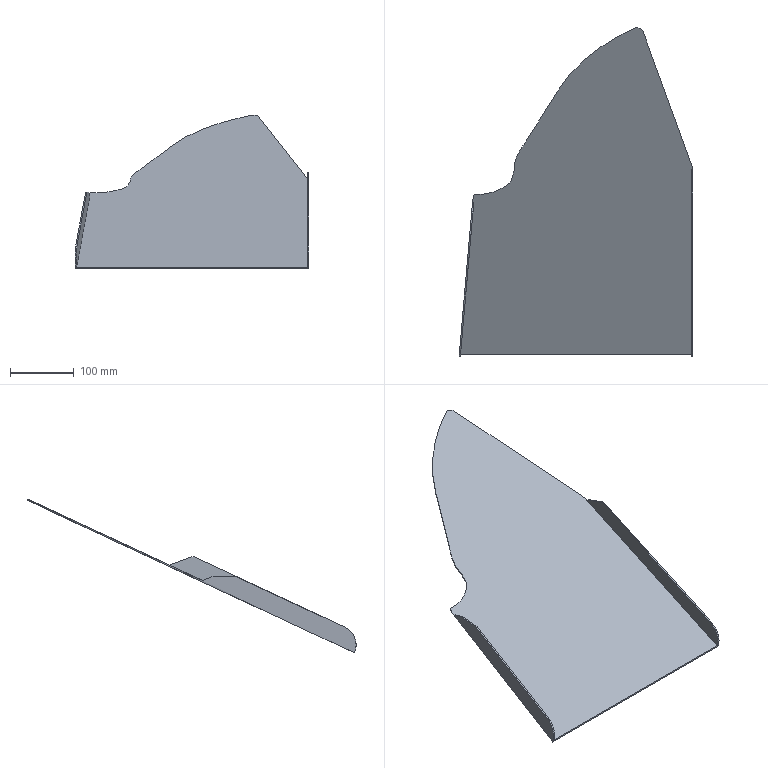Part | NX | features solid 2 | 1 solid | 19 faces | box 365.998 x 513.743 x 240.459 mm | volume 359424 mm3 | plane 12 | spline 4 | cylinder 3 | commonest cylinder face diameters 60 x2 20 x1
STEP:
#1=CARTESIAN_POINT('',(-655.461,-379.114,-82.467));
#2=VERTEX_POINT('',#1);
#3=CARTESIAN_POINT('',(-827.658,-589.836,-180.722));
#4=VERTEX_POINT('',#3);
#5=CARTESIAN_POINT('',(-655.471,-379.107,-82.458));
#6=CARTESIAN_POINT('',(-660.107,-383.195,-84.364));
#7=CARTESIAN_POINT('',(-669.009,-391.621,-88.293));
#8=CARTESIAN_POINT('',(-681.292,-404.984,-94.524));
#9=CARTESIAN_POINT('',(-692.185,-419.286,-101.194));
#10=CARTESIAN_POINT('',(-701.759,-434.482,-108.279));
#11=CARTESIAN_POINT('',(-711.123,-449.816,-115.43));
#12=CARTESIAN_POINT('',(-720.618,-465.075,-122.545));
#13=CARTESIAN_POINT('',(-730.26,-480.26,-129.626));
#14=CARTESIAN_POINT('',(-738.35,-492.885,-135.513));
#15=CARTESIAN_POINT('',(-744.785,-503.005,-140.232));
#16=CARTESIAN_POINT('',(-749.566,-510.617,-143.782));
#17=CARTESIAN_POINT('',(-753.85,-516.81,-146.669));
#18=CARTESIAN_POINT('',(-757.144,-521.829,-149.01));
#19=CARTESIAN_POINT('',(-759.928,-527.088,-151.462));
#20=CARTESIAN_POINT('',(-762.27,-532.572,-154.02));
#21=CARTESIAN_POINT('',(-764.142,-537.399,-156.271));
#22=CARTESIAN_POINT('',(-764.925,-540.201,-157.577));
#23=CARTESIAN_POINT('',(-765.338,-542.328,-158.569));
#24=CARTESIAN_POINT('',(-765.394,-543.962,-159.331));
#25=CARTESIAN_POINT('',(-765.323,-545.068,-159.846));
#26=CARTESIAN_POINT('',(-765.221,-545.813,-160.194));
#27=CARTESIAN_POINT('',(-765.171,-547.827,-161.133));
#28=CARTESIAN_POINT('',(-764.947,-550.426,-162.345));
#29=CARTESIAN_POINT('',(-765.798,-553.164,-163.622));
#30=CARTESIAN_POINT('',(-766.616,-555.908,-164.901));
#31=CARTESIAN_POINT('',(-767.546,-559.361,-166.511));
#32=CARTESIAN_POINT('',(-768.584,-563.51,-168.446));
#33=CARTESIAN_POINT('',(-769.892,-567.64,-170.372));
#34=CARTESIAN_POINT('',(-772.053,-571.414,-172.132));
#35=CARTESIAN_POINT('',(-775.516,-574.418,-173.533));
#36=CARTESIAN_POINT('',(-779.232,-576.955,-174.716));
#37=CARTESIAN_POINT('',(-784.427,-580.123,-176.193));
#38=CARTESIAN_POINT('',(-791.252,-583.583,-177.806));
#39=CARTESIAN_POINT('',(-799.806,-586.768,-179.292));
#40=CARTESIAN_POINT('',(-808.892,-588.923,-180.297));
#41=CARTESIAN_POINT('',(-816.696,-589.681,-180.65));
#42=CARTESIAN_POINT('',(-822.96,-589.749,-180.682));
#43=CARTESIAN_POINT('',(-826.092,-589.809,-180.71));
#44=CARTESIAN_POINT('',(-827.658,-589.836,-180.722));
#45=B_SPLINE_CURVE_WITH_KNOTS('',3,(#5,#6,#7,#8,#9,#10,#11,#12,#13,#14,#15,#16,#17,#18,#19,#20,#21,#22,#23,#24,#25,#26,#27,#28,#29,#30,#31,#32,#33,#34,#35,#36,#37,#38,#39,#40,#41,#42,#43,#44),.UNSPECIFIED.,.F.,.F.,(4,1,1,1,1,1,1,1,1,1,1,1,1,1,1,1,1,1,1,1,1,1,1,1,1,1,1,1,1,1,1,1,1,1,1,1,1,4),(0.00205,0.02121,0.04038,0.05954,0.0787,0.09786,0.117,0.1362,0.1554,0.1649,0.1745,0.1841,0.1889,0.1937,0.2033,0.208,0.2104,0.2128,0.2152,0.2158,0.2164,0.2176,0.2224,0.2248,0.2272,0.232,0.2368,0.2416,0.2464,0.2512,0.256,0.2607,0.2703,0.2799,0.2895,0.2991,0.3039,0.3087),.UNSPECIFIED.);
#46=EDGE_CURVE('',#2,#4,#45,.T.);
#47=ORIENTED_EDGE('',*,*,#46,.T.);
#48=CARTESIAN_POINT('',(-830.649,-601.717,-186.262));
#49=VERTEX_POINT('',#48);
#50=CARTESIAN_POINT('',(-827.658,-589.836,-180.722));
#51=CARTESIAN_POINT('',(-828.837,-591.553,-181.523));
#52=CARTESIAN_POINT('',(-830.427,-595.498,-183.362));
#53=CARTESIAN_POINT('',(-830.5,-599.654,-185.3));
#54=CARTESIAN_POINT('',(-830.649,-601.717,-186.262));
#55=B_SPLINE_CURVE_WITH_KNOTS('',3,(#50,#51,#52,#53,#54),.UNSPECIFIED.,.F.,.F.,(4,1,4),(0.8418,0.8485,0.8553),.UNSPECIFIED.);
#56=EDGE_CURVE('',#4,#49,#55,.T.);
#57=ORIENTED_EDGE('',*,*,#56,.T.);
#58=CARTESIAN_POINT('',(-828.644,-601.717,-186.262));
#59=VERTEX_POINT('',#58);
#60=CARTESIAN_POINT('',(-750.,-601.717,-186.262));
#61=DIRECTION('',(-1.,0.,0.));
#62=VECTOR('',#61,1000.);
#63=LINE('',#60,#62);
#64=EDGE_CURVE('',#49,#59,#63,.F.);
#65=ORIENTED_EDGE('',*,*,#64,.T.);
#66=CARTESIAN_POINT('',(-849.475,-840.,-297.376));
#67=VERTEX_POINT('',#66);
#68=CARTESIAN_POINT('',(-849.475,-840.,-297.376));
#69=CARTESIAN_POINT('',(-847.736,-820.143,-288.116));
#70=CARTESIAN_POINT('',(-844.258,-780.43,-269.597));
#71=CARTESIAN_POINT('',(-839.91,-730.788,-246.449));
#72=CARTESIAN_POINT('',(-836.432,-691.074,-227.93));
#73=CARTESIAN_POINT('',(-833.824,-661.289,-214.041));
#74=CARTESIAN_POINT('',(-831.657,-636.468,-202.467));
#75=CARTESIAN_POINT('',(-830.132,-619.094,-194.365));
#76=CARTESIAN_POINT('',(-829.284,-609.164,-189.735));
#77=CARTESIAN_POINT('',(-828.821,-604.201,-187.421));
#78=CARTESIAN_POINT('',(-828.644,-601.717,-186.262));
#79=B_SPLINE_CURVE_WITH_KNOTS('',3,(#68,#69,#70,#71,#72,#73,#74,#75,#76,#77,#78),.UNSPECIFIED.,.F.,.F.,(4,1,1,1,1,1,1,1,4),(0.6332,0.6991,0.7651,0.7981,0.831,0.864,0.8805,0.8887,0.897),.UNSPECIFIED.);
#80=EDGE_CURVE('',#59,#67,#79,.F.);
#81=ORIENTED_EDGE('',*,*,#80,.T.);
#82=CARTESIAN_POINT('',(-487.731,-840.,-297.376));
#83=VERTEX_POINT('',#82);
#84=CARTESIAN_POINT('',(-1209.175,-840.,-297.376));
#85=DIRECTION('',(-1.,0.,0.));
#86=VECTOR('',#85,1000.);
#87=LINE('',#84,#86);
#88=EDGE_CURVE('',#67,#83,#87,.F.);
#89=ORIENTED_EDGE('',*,*,#88,.T.);
#90=CARTESIAN_POINT('',(-487.731,-550.363,-162.315));
#91=VERTEX_POINT('',#90);
#92=CARTESIAN_POINT('',(-487.731,-651.161,-209.318));
#93=DIRECTION('',(0.,-0.9063,-0.4226));
#94=VECTOR('',#93,1000.);
#95=LINE('',#92,#94);
#96=EDGE_CURVE('',#91,#83,#95,.T.);
#97=ORIENTED_EDGE('',*,*,#96,.F.);
#98=CARTESIAN_POINT('',(-485.731,-550.363,-162.315));
#99=VERTEX_POINT('',#98);
#100=CARTESIAN_POINT('',(-485.731,-550.363,-162.315));
#101=DIRECTION('',(1.,0.,0.));
#102=VECTOR('',#101,1000.);
#103=LINE('',#100,#102);
#104=EDGE_CURVE('',#91,#99,#103,.T.);
#105=ORIENTED_EDGE('',*,*,#104,.T.);
#106=CARTESIAN_POINT('',(-485.731,-549.517,-161.921));
#107=VERTEX_POINT('',#106);
#108=CARTESIAN_POINT('',(-485.731,-651.161,-209.318));
#109=DIRECTION('',(0.,-0.9063,-0.4226));
#110=VECTOR('',#109,1000.);
#111=LINE('',#108,#110);
#112=EDGE_CURVE('',#107,#99,#111,.T.);
#113=ORIENTED_EDGE('',*,*,#112,.F.);
#114=CARTESIAN_POINT('',(-563.574,-335.647,-62.192));
#115=VERTEX_POINT('',#114);
#116=CARTESIAN_POINT('',(-523.362,-446.128,-113.71));
#117=DIRECTION('',(-0.3133,0.8607,0.4013));
#118=VECTOR('',#117,1000.);
#119=LINE('',#116,#118);
#120=EDGE_CURVE('',#107,#115,#119,.T.);
#121=ORIENTED_EDGE('',*,*,#120,.T.);
#122=CARTESIAN_POINT('',(-576.985,-329.909,-59.516));
#123=VERTEX_POINT('',#122);
#124=CARTESIAN_POINT('',(-572.971,-339.067,-63.787));
#125=DIRECTION('',(0.,-0.4226,0.9063));
#126=DIRECTION('',(0.,-0.9063,-0.4226));
#127=AXIS2_PLACEMENT_3D('',#124,#125,#126);
#128=ELLIPSE('',#127,11.034,10.);
#129=EDGE_CURVE('',#115,#123,#128,.T.);
#130=ORIENTED_EDGE('',*,*,#129,.T.);
#131=CARTESIAN_POINT('',(-655.461,-379.14,-82.473));
#132=CARTESIAN_POINT('',(-643.996,-369.015,-77.752));
#133=CARTESIAN_POINT('',(-625.37,-355.322,-71.366));
#134=CARTESIAN_POINT('',(-598.375,-339.759,-64.11));
#135=CARTESIAN_POINT('',(-584.188,-333.066,-60.988));
#136=CARTESIAN_POINT('',(-576.985,-329.909,-59.516));
#137=B_SPLINE_CURVE_WITH_KNOTS('',3,(#131,#132,#133,#134,#135,#136),.UNSPECIFIED.,.F.,.F.,(4,1,1,4),(0.0008076,0.04866,0.07259,0.09652),.UNSPECIFIED.);
#138=EDGE_CURVE('',#2,#123,#137,.T.);
#139=ORIENTED_EDGE('',*,*,#138,.F.);
#140=EDGE_LOOP('',(#47,#57,#65,#81,#89,#97,#105,#113,#121,#130,#139));
#141=FACE_BOUND('',#140,.T.);
#142=CARTESIAN_POINT('',(-1209.175,-651.161,-209.318));
#143=DIRECTION('',(0.,-0.4226,0.9063));
#144=DIRECTION('',(1.,0.,0.));
#145=AXIS2_PLACEMENT_3D('',#142,#143,#144);
#146=PLANE('',#145);
#147=ADVANCED_FACE('',(#141),#146,.T.);
#148=CARTESIAN_POINT('',(-827.658,-589.836,-182.929));
#149=VERTEX_POINT('',#148);
#150=CARTESIAN_POINT('',(-851.483,-840.,-299.582));
#151=VERTEX_POINT('',#150);
#152=CARTESIAN_POINT('',(-827.658,-589.836,-182.929));
#153=CARTESIAN_POINT('',(-828.455,-590.997,-183.47));
#154=CARTESIAN_POINT('',(-829.702,-593.543,-184.658));
#155=CARTESIAN_POINT('',(-830.416,-597.398,-186.455));
#156=CARTESIAN_POINT('',(-830.592,-601.333,-188.29));
#157=CARTESIAN_POINT('',(-830.944,-605.243,-190.113));
#158=CARTESIAN_POINT('',(-831.281,-609.157,-191.938));
#159=CARTESIAN_POINT('',(-831.735,-614.374,-194.371));
#160=CARTESIAN_POINT('',(-832.302,-620.895,-197.412));
#161=CARTESIAN_POINT('',(-832.985,-628.72,-201.061));
#162=CARTESIAN_POINT('',(-833.896,-639.154,-205.926));
#163=CARTESIAN_POINT('',(-835.037,-652.196,-212.008));
#164=CARTESIAN_POINT('',(-836.406,-667.846,-219.306));
#165=CARTESIAN_POINT('',(-837.776,-683.497,-226.604));
#166=CARTESIAN_POINT('',(-839.147,-699.147,-233.902));
#167=CARTESIAN_POINT('',(-840.975,-720.014,-243.632));
#168=CARTESIAN_POINT('',(-843.259,-746.098,-255.795));
#169=CARTESIAN_POINT('',(-846.,-777.399,-270.391));
#170=CARTESIAN_POINT('',(-848.742,-808.699,-284.987));
#171=CARTESIAN_POINT('',(-850.569,-829.566,-294.717));
#172=CARTESIAN_POINT('',(-851.483,-840.,-299.582));
#173=B_SPLINE_CURVE_WITH_KNOTS('',3,(#152,#153,#154,#155,#156,#157,#158,#159,#160,#161,#162,#163,#164,#165,#166,#167,#168,#169,#170,#171,#172),.UNSPECIFIED.,.F.,.F.,(4,1,1,1,1,1,1,1,1,1,1,1,1,1,1,1,1,1,4),(0.1708,0.1753,0.1799,0.1844,0.1889,0.1934,0.1979,0.2069,0.2159,0.2249,0.2429,0.261,0.279,0.297,0.315,0.3511,0.3871,0.4232,0.4592),.UNSPECIFIED.);
#174=EDGE_CURVE('',#149,#151,#173,.T.);
#175=ORIENTED_EDGE('',*,*,#174,.F.);
#176=CARTESIAN_POINT('',(-655.461,-379.114,-84.674));
#177=VERTEX_POINT('',#176);
#178=CARTESIAN_POINT('',(-655.471,-379.107,-84.664));
#179=CARTESIAN_POINT('',(-660.107,-383.195,-86.571));
#180=CARTESIAN_POINT('',(-669.009,-391.621,-90.5));
#181=CARTESIAN_POINT('',(-681.292,-404.984,-96.731));
#182=CARTESIAN_POINT('',(-692.185,-419.286,-103.4));
#183=CARTESIAN_POINT('',(-701.759,-434.482,-110.486));
#184=CARTESIAN_POINT('',(-711.123,-449.816,-117.636));
#185=CARTESIAN_POINT('',(-720.618,-465.075,-124.752));
#186=CARTESIAN_POINT('',(-730.26,-480.26,-131.833));
#187=CARTESIAN_POINT('',(-738.35,-492.885,-137.72));
#188=CARTESIAN_POINT('',(-744.785,-503.005,-142.439));
#189=CARTESIAN_POINT('',(-749.566,-510.617,-145.989));
#190=CARTESIAN_POINT('',(-753.85,-516.81,-148.876));
#191=CARTESIAN_POINT('',(-757.144,-521.829,-151.217));
#192=CARTESIAN_POINT('',(-759.928,-527.088,-153.669));
#193=CARTESIAN_POINT('',(-762.27,-532.572,-156.226));
#194=CARTESIAN_POINT('',(-764.142,-537.399,-158.477));
#195=CARTESIAN_POINT('',(-764.925,-540.201,-159.784));
#196=CARTESIAN_POINT('',(-765.338,-542.328,-160.776));
#197=CARTESIAN_POINT('',(-765.394,-543.962,-161.538));
#198=CARTESIAN_POINT('',(-765.323,-545.068,-162.053));
#199=CARTESIAN_POINT('',(-765.221,-545.813,-162.401));
#200=CARTESIAN_POINT('',(-765.171,-547.827,-163.34));
#201=CARTESIAN_POINT('',(-764.947,-550.426,-164.552));
#202=CARTESIAN_POINT('',(-765.798,-553.164,-165.829));
#203=CARTESIAN_POINT('',(-766.616,-555.908,-167.108));
#204=CARTESIAN_POINT('',(-767.546,-559.361,-168.718));
#205=CARTESIAN_POINT('',(-768.584,-563.51,-170.653));
#206=CARTESIAN_POINT('',(-769.892,-567.64,-172.579));
#207=CARTESIAN_POINT('',(-772.053,-571.414,-174.339));
#208=CARTESIAN_POINT('',(-775.516,-574.418,-175.74));
#209=CARTESIAN_POINT('',(-779.232,-576.955,-176.923));
#210=CARTESIAN_POINT('',(-784.427,-580.123,-178.4));
#211=CARTESIAN_POINT('',(-791.252,-583.583,-180.013));
#212=CARTESIAN_POINT('',(-799.806,-586.768,-181.498));
#213=CARTESIAN_POINT('',(-808.892,-588.923,-182.503));
#214=CARTESIAN_POINT('',(-816.696,-589.681,-182.857));
#215=CARTESIAN_POINT('',(-822.96,-589.749,-182.888));
#216=CARTESIAN_POINT('',(-826.092,-589.809,-182.917));
#217=CARTESIAN_POINT('',(-827.658,-589.836,-182.929));
#218=B_SPLINE_CURVE_WITH_KNOTS('',3,(#178,#179,#180,#181,#182,#183,#184,#185,#186,#187,#188,#189,#190,#191,#192,#193,#194,#195,#196,#197,#198,#199,#200,#201,#202,#203,#204,#205,#206,#207,#208,#209,#210,#211,#212,#213,#214,#215,#216,#217),.UNSPECIFIED.,.F.,.F.,(4,1,1,1,1,1,1,1,1,1,1,1,1,1,1,1,1,1,1,1,1,1,1,1,1,1,1,1,1,1,1,1,1,1,1,1,1,4),(0.00205,0.02121,0.04038,0.05954,0.0787,0.09786,0.117,0.1362,0.1554,0.1649,0.1745,0.1841,0.1889,0.1937,0.2033,0.208,0.2104,0.2128,0.2152,0.2158,0.2164,0.2176,0.2224,0.2248,0.2272,0.232,0.2368,0.2416,0.2464,0.2512,0.256,0.2607,0.2703,0.2799,0.2895,0.2991,0.3039,0.3087),.UNSPECIFIED.);
#219=EDGE_CURVE('',#177,#149,#218,.T.);
#220=ORIENTED_EDGE('',*,*,#219,.F.);
#221=CARTESIAN_POINT('',(-576.985,-329.909,-61.723));
#222=VERTEX_POINT('',#221);
#223=CARTESIAN_POINT('',(-655.461,-379.14,-84.68));
#224=CARTESIAN_POINT('',(-643.996,-369.015,-79.958));
#225=CARTESIAN_POINT('',(-625.37,-355.322,-73.573));
#226=CARTESIAN_POINT('',(-598.375,-339.759,-66.316));
#227=CARTESIAN_POINT('',(-584.188,-333.066,-63.195));
#228=CARTESIAN_POINT('',(-576.985,-329.909,-61.723));
#229=B_SPLINE_CURVE_WITH_KNOTS('',3,(#223,#224,#225,#226,#227,#228),.UNSPECIFIED.,.F.,.F.,(4,1,1,4),(0.0008076,0.04866,0.07259,0.09652),.UNSPECIFIED.);
#230=EDGE_CURVE('',#177,#222,#229,.T.);
#231=ORIENTED_EDGE('',*,*,#230,.T.);
#232=CARTESIAN_POINT('',(-563.574,-335.647,-64.399));
#233=VERTEX_POINT('',#232);
#234=CARTESIAN_POINT('',(-572.971,-339.067,-65.994));
#235=DIRECTION('',(0.,-0.4226,0.9063));
#236=DIRECTION('',(0.,-0.9063,-0.4226));
#237=AXIS2_PLACEMENT_3D('',#234,#235,#236);
#238=ELLIPSE('',#237,11.034,10.);
#239=EDGE_CURVE('',#222,#233,#238,.F.);
#240=ORIENTED_EDGE('',*,*,#239,.T.);
#241=CARTESIAN_POINT('',(-485.731,-549.517,-164.128));
#242=VERTEX_POINT('',#241);
#243=CARTESIAN_POINT('',(-523.639,-445.366,-115.561));
#244=DIRECTION('',(-0.3133,0.8607,0.4013));
#245=VECTOR('',#244,1000.);
#246=LINE('',#243,#245);
#247=EDGE_CURVE('',#242,#233,#246,.T.);
#248=ORIENTED_EDGE('',*,*,#247,.F.);
#249=CARTESIAN_POINT('',(-485.731,-840.,-299.582));
#250=VERTEX_POINT('',#249);
#251=CARTESIAN_POINT('',(-485.731,-650.315,-211.131));
#252=DIRECTION('',(0.,-0.9063,-0.4226));
#253=VECTOR('',#252,1000.);
#254=LINE('',#251,#253);
#255=EDGE_CURVE('',#242,#250,#254,.T.);
#256=ORIENTED_EDGE('',*,*,#255,.T.);
#257=CARTESIAN_POINT('',(-487.731,-840.,-299.582));
#258=VERTEX_POINT('',#257);
#259=CARTESIAN_POINT('',(-485.731,-840.,-299.582));
#260=DIRECTION('',(1.,0.,0.));
#261=VECTOR('',#260,1000.);
#262=LINE('',#259,#261);
#263=EDGE_CURVE('',#250,#258,#262,.F.);
#264=ORIENTED_EDGE('',*,*,#263,.T.);
#265=CARTESIAN_POINT('',(-849.475,-840.,-299.582));
#266=VERTEX_POINT('',#265);
#267=CARTESIAN_POINT('',(-1209.175,-840.,-299.582));
#268=DIRECTION('',(-1.,0.,0.));
#269=VECTOR('',#268,1000.);
#270=LINE('',#267,#269);
#271=EDGE_CURVE('',#266,#258,#270,.F.);
#272=ORIENTED_EDGE('',*,*,#271,.F.);
#273=CARTESIAN_POINT('',(-1209.175,-840.,-299.582));
#274=DIRECTION('',(-1.,0.,0.));
#275=VECTOR('',#274,1000.);
#276=LINE('',#273,#275);
#277=EDGE_CURVE('',#151,#266,#276,.F.);
#278=ORIENTED_EDGE('',*,*,#277,.F.);
#279=EDGE_LOOP('',(#175,#220,#231,#240,#248,#256,#264,#272,#278));
#280=FACE_BOUND('',#279,.T.);
#281=CARTESIAN_POINT('',(-1209.175,-650.315,-211.131));
#282=DIRECTION('',(0.,-0.4226,0.9063));
#283=DIRECTION('',(1.,0.,0.));
#284=AXIS2_PLACEMENT_3D('',#281,#282,#283);
#285=PLANE('',#284);
#286=ADVANCED_FACE('',(#280),#285,.F.);
#287=ORIENTED_EDGE('',*,*,#56,.F.);
#288=CARTESIAN_POINT('',(-827.658,-589.836,-182.929));
#289=DIRECTION('',(0.,0.,-1.));
#290=VECTOR('',#289,1000.);
#291=LINE('',#288,#290);
#292=EDGE_CURVE('',#149,#4,#291,.F.);
#293=ORIENTED_EDGE('',*,*,#292,.F.);
#294=ORIENTED_EDGE('',*,*,#174,.T.);
#295=CARTESIAN_POINT('',(-850.212,-825.489,-259.715));
#296=VERTEX_POINT('',#295);
#297=CARTESIAN_POINT('',(-851.483,-840.,-299.582));
#298=CARTESIAN_POINT('',(-851.555,-840.826,-297.811));
#299=CARTESIAN_POINT('',(-851.671,-842.145,-294.05));
#300=CARTESIAN_POINT('',(-851.768,-843.254,-286.301));
#301=CARTESIAN_POINT('',(-851.633,-841.716,-276.296));
#302=CARTESIAN_POINT('',(-851.087,-835.481,-266.094));
#303=CARTESIAN_POINT('',(-850.522,-829.027,-261.364));
#304=CARTESIAN_POINT('',(-850.212,-825.489,-259.715));
#305=B_SPLINE_CURVE_WITH_KNOTS('',3,(#297,#298,#299,#300,#301,#302,#303,#304),.UNSPECIFIED.,.F.,.F.,(4,1,1,1,1,4),(0.1679,0.1738,0.1796,0.1913,0.2031,0.2148),.UNSPECIFIED.);
#306=EDGE_CURVE('',#151,#296,#305,.T.);
#307=ORIENTED_EDGE('',*,*,#306,.T.);
#308=CARTESIAN_POINT('',(-835.242,-654.541,-180.));
#309=VERTEX_POINT('',#308);
#310=CARTESIAN_POINT('',(-850.212,-825.489,-259.715));
#311=CARTESIAN_POINT('',(-845.221,-768.507,-233.143));
#312=CARTESIAN_POINT('',(-840.227,-711.524,-206.572));
#313=CARTESIAN_POINT('',(-835.242,-654.541,-180.));
#314=B_SPLINE_CURVE_WITH_KNOTS('',3,(#310,#311,#312,#313),.UNSPECIFIED.,.F.,.F.,(4,4),(1.624,1.814),.UNSPECIFIED.);
#315=EDGE_CURVE('',#309,#296,#314,.F.);
#316=ORIENTED_EDGE('',*,*,#315,.F.);
#317=CARTESIAN_POINT('',(-832.131,-618.922,-180.));
#318=VERTEX_POINT('',#317);
#319=CARTESIAN_POINT('',(-832.131,-618.922,-180.));
#320=CARTESIAN_POINT('',(-833.165,-630.795,-180.));
#321=CARTESIAN_POINT('',(-834.204,-642.668,-180.));
#322=CARTESIAN_POINT('',(-835.242,-654.541,-180.));
#323=B_SPLINE_CURVE_WITH_KNOTS('',3,(#319,#320,#321,#322),.UNSPECIFIED.,.F.,.F.,(4,4),(0.1911,0.2274),.UNSPECIFIED.);
#324=EDGE_CURVE('',#318,#309,#323,.T.);
#325=ORIENTED_EDGE('',*,*,#324,.F.);
#326=CARTESIAN_POINT('',(-832.131,-618.922,-180.));
#327=CARTESIAN_POINT('',(-831.881,-616.054,-181.044));
#328=CARTESIAN_POINT('',(-831.396,-610.319,-183.131));
#329=CARTESIAN_POINT('',(-830.856,-604.587,-185.217));
#330=CARTESIAN_POINT('',(-830.649,-601.717,-186.262));
#331=B_SPLINE_CURVE_WITH_KNOTS('',3,(#326,#327,#328,#329,#330),.UNSPECIFIED.,.F.,.F.,(4,1,4),(0.08658,0.09577,0.105),.UNSPECIFIED.);
#332=EDGE_CURVE('',#318,#49,#331,.T.);
#333=ORIENTED_EDGE('',*,*,#332,.T.);
#334=EDGE_LOOP('',(#287,#293,#294,#307,#316,#325,#333));
#335=FACE_BOUND('',#334,.T.);
#336=CARTESIAN_POINT('',(-827.658,-589.836,-300.3));
#337=CARTESIAN_POINT('',(-827.658,-589.836,-180.));
#338=CARTESIAN_POINT('',(-828.212,-590.643,-300.3));
#339=CARTESIAN_POINT('',(-828.212,-590.643,-180.));
#340=CARTESIAN_POINT('',(-828.914,-591.92,-300.3));
#341=CARTESIAN_POINT('',(-828.914,-591.92,-180.));
#342=CARTESIAN_POINT('',(-829.589,-593.726,-300.3));
#343=CARTESIAN_POINT('',(-829.589,-593.726,-180.));
#344=CARTESIAN_POINT('',(-829.905,-594.856,-300.3));
#345=CARTESIAN_POINT('',(-829.905,-594.856,-180.));
#346=CARTESIAN_POINT('',(-830.112,-595.859,-300.3));
#347=CARTESIAN_POINT('',(-830.112,-595.859,-180.));
#348=CARTESIAN_POINT('',(-830.21,-596.458,-300.3));
#349=CARTESIAN_POINT('',(-830.21,-596.458,-180.));
#350=CARTESIAN_POINT('',(-830.331,-597.38,-300.3));
#351=CARTESIAN_POINT('',(-830.331,-597.38,-180.));
#352=CARTESIAN_POINT('',(-830.421,-598.38,-300.3));
#353=CARTESIAN_POINT('',(-830.421,-598.38,-180.));
#354=CARTESIAN_POINT('',(-830.477,-599.132,-300.3));
#355=CARTESIAN_POINT('',(-830.477,-599.132,-180.));
#356=CARTESIAN_POINT('',(-830.509,-599.627,-300.3));
#357=CARTESIAN_POINT('',(-830.509,-599.627,-180.));
#358=CARTESIAN_POINT('',(-830.541,-600.139,-300.3));
#359=CARTESIAN_POINT('',(-830.541,-600.139,-180.));
#360=CARTESIAN_POINT('',(-830.592,-600.909,-300.3));
#361=CARTESIAN_POINT('',(-830.592,-600.909,-180.));
#362=CARTESIAN_POINT('',(-830.648,-601.707,-300.3));
#363=CARTESIAN_POINT('',(-830.648,-601.707,-180.));
#364=CARTESIAN_POINT('',(-830.687,-602.241,-300.3));
#365=CARTESIAN_POINT('',(-830.687,-602.241,-180.));
#366=CARTESIAN_POINT('',(-830.711,-602.543,-300.3));
#367=CARTESIAN_POINT('',(-830.711,-602.543,-180.));
#368=CARTESIAN_POINT('',(-830.724,-602.719,-300.3));
#369=CARTESIAN_POINT('',(-830.724,-602.719,-180.));
#370=CARTESIAN_POINT('',(-830.737,-602.88,-300.3));
#371=CARTESIAN_POINT('',(-830.737,-602.88,-180.));
#372=CARTESIAN_POINT('',(-830.734,-602.835,-300.3));
#373=CARTESIAN_POINT('',(-830.734,-602.835,-180.));
#374=CARTESIAN_POINT('',(-830.737,-602.877,-300.3));
#375=CARTESIAN_POINT('',(-830.737,-602.877,-180.));
#376=CARTESIAN_POINT('',(-830.742,-602.932,-300.3));
#377=CARTESIAN_POINT('',(-830.742,-602.932,-180.));
#378=CARTESIAN_POINT('',(-830.76,-603.142,-300.3));
#379=CARTESIAN_POINT('',(-830.76,-603.142,-180.));
#380=CARTESIAN_POINT('',(-830.803,-603.648,-300.3));
#381=CARTESIAN_POINT('',(-830.803,-603.648,-180.));
#382=CARTESIAN_POINT('',(-830.89,-604.644,-300.3));
#383=CARTESIAN_POINT('',(-830.89,-604.644,-180.));
#384=CARTESIAN_POINT('',(-831.042,-606.403,-300.3));
#385=CARTESIAN_POINT('',(-831.042,-606.403,-180.));
#386=CARTESIAN_POINT('',(-831.211,-608.342,-300.3));
#387=CARTESIAN_POINT('',(-831.211,-608.342,-180.));
#388=CARTESIAN_POINT('',(-831.37,-610.177,-300.3));
#389=CARTESIAN_POINT('',(-831.37,-610.177,-180.));
#390=CARTESIAN_POINT('',(-831.502,-611.693,-300.3));
#391=CARTESIAN_POINT('',(-831.502,-611.693,-180.));
#392=CARTESIAN_POINT('',(-831.622,-613.079,-300.3));
#393=CARTESIAN_POINT('',(-831.622,-613.079,-180.));
#394=CARTESIAN_POINT('',(-831.724,-614.249,-300.3));
#395=CARTESIAN_POINT('',(-831.724,-614.249,-180.));
#396=CARTESIAN_POINT('',(-831.792,-615.033,-300.3));
#397=CARTESIAN_POINT('',(-831.792,-615.033,-180.));
#398=CARTESIAN_POINT('',(-831.837,-615.55,-300.3));
#399=CARTESIAN_POINT('',(-831.837,-615.55,-180.));
#400=CARTESIAN_POINT('',(-831.87,-615.923,-300.3));
#401=CARTESIAN_POINT('',(-831.87,-615.923,-180.));
#402=CARTESIAN_POINT('',(-831.878,-616.023,-300.3));
#403=CARTESIAN_POINT('',(-831.878,-616.023,-180.));
#404=CARTESIAN_POINT('',(-831.892,-616.178,-300.3));
#405=CARTESIAN_POINT('',(-831.892,-616.178,-180.));
#406=CARTESIAN_POINT('',(-831.912,-616.41,-300.3));
#407=CARTESIAN_POINT('',(-831.912,-616.41,-180.));
#408=CARTESIAN_POINT('',(-831.938,-616.71,-300.3));
#409=CARTESIAN_POINT('',(-831.938,-616.71,-180.));
#410=CARTESIAN_POINT('',(-832.001,-617.436,-300.3));
#411=CARTESIAN_POINT('',(-832.001,-617.436,-180.));
#412=CARTESIAN_POINT('',(-832.1,-618.568,-300.3));
#413=CARTESIAN_POINT('',(-832.1,-618.568,-180.));
#414=CARTESIAN_POINT('',(-832.239,-620.163,-300.3));
#415=CARTESIAN_POINT('',(-832.239,-620.163,-180.));
#416=CARTESIAN_POINT('',(-832.434,-622.406,-300.3));
#417=CARTESIAN_POINT('',(-832.434,-622.406,-180.));
#418=CARTESIAN_POINT('',(-832.697,-625.426,-300.3));
#419=CARTESIAN_POINT('',(-832.697,-625.426,-180.));
#420=CARTESIAN_POINT('',(-833.045,-629.403,-300.3));
#421=CARTESIAN_POINT('',(-833.045,-629.403,-180.));
#422=CARTESIAN_POINT('',(-833.421,-633.712,-300.3));
#423=CARTESIAN_POINT('',(-833.421,-633.712,-180.));
#424=CARTESIAN_POINT('',(-833.764,-637.641,-300.3));
#425=CARTESIAN_POINT('',(-833.764,-637.641,-180.));
#426=CARTESIAN_POINT('',(-834.01,-640.45,-300.3));
#427=CARTESIAN_POINT('',(-834.01,-640.45,-180.));
#428=CARTESIAN_POINT('',(-834.167,-642.245,-300.3));
#429=CARTESIAN_POINT('',(-834.167,-642.245,-180.));
#430=CARTESIAN_POINT('',(-834.272,-643.443,-300.3));
#431=CARTESIAN_POINT('',(-834.272,-643.443,-180.));
#432=CARTESIAN_POINT('',(-834.42,-645.144,-300.3));
#433=CARTESIAN_POINT('',(-834.42,-645.144,-180.));
#434=CARTESIAN_POINT('',(-834.649,-647.752,-300.3));
#435=CARTESIAN_POINT('',(-834.649,-647.752,-180.));
#436=CARTESIAN_POINT('',(-834.937,-651.052,-300.3));
#437=CARTESIAN_POINT('',(-834.937,-651.052,-180.));
#438=CARTESIAN_POINT('',(-835.397,-656.308,-300.3));
#439=CARTESIAN_POINT('',(-835.397,-656.308,-180.));
#440=CARTESIAN_POINT('',(-835.973,-662.887,-300.3));
#441=CARTESIAN_POINT('',(-835.973,-662.887,-180.));
#442=CARTESIAN_POINT('',(-836.893,-673.409,-300.3));
#443=CARTESIAN_POINT('',(-836.893,-673.409,-180.));
#444=CARTESIAN_POINT('',(-838.045,-686.562,-300.3));
#445=CARTESIAN_POINT('',(-838.045,-686.562,-180.));
#446=CARTESIAN_POINT('',(-839.427,-702.345,-300.3));
#447=CARTESIAN_POINT('',(-839.427,-702.345,-180.));
#448=CARTESIAN_POINT('',(-841.27,-723.39,-300.3));
#449=CARTESIAN_POINT('',(-841.27,-723.39,-180.));
#450=CARTESIAN_POINT('',(-843.574,-749.696,-300.3));
#451=CARTESIAN_POINT('',(-843.574,-749.696,-180.));
#452=CARTESIAN_POINT('',(-846.339,-781.263,-300.3));
#453=CARTESIAN_POINT('',(-846.339,-781.263,-180.));
#454=CARTESIAN_POINT('',(-849.103,-812.831,-300.3));
#455=CARTESIAN_POINT('',(-849.103,-812.831,-180.));
#456=CARTESIAN_POINT('',(-850.946,-833.875,-300.3));
#457=CARTESIAN_POINT('',(-850.946,-833.875,-180.));
#458=CARTESIAN_POINT('',(-851.868,-844.398,-300.3));
#459=CARTESIAN_POINT('',(-851.868,-844.398,-180.));
#460=B_SPLINE_SURFACE_WITH_KNOTS('',3,1,((#336,#337),(#338,#339),(#340,#341),(#342,#343),(#344,#345),(#346,#347),(#348,#349),(#350,#351),(#352,#353),(#354,#355),(#356,#357),(#358,#359),(#360,#361),(#362,#363),(#364,#365),(#366,#367),(#368,#369),(#370,#371),(#372,#373),(#374,#375),(#376,#377),(#378,#379),(#380,#381),(#382,#383),(#384,#385),(#386,#387),(#388,#389),(#390,#391),(#392,#393),(#394,#395),(#396,#397),(#398,#399),(#400,#401),(#402,#403),(#404,#405),(#406,#407),(#408,#409),(#410,#411),(#412,#413),(#414,#415),(#416,#417),(#418,#419),(#420,#421),(#422,#423),(#424,#425),(#426,#427),(#428,#429),(#430,#431),(#432,#433),(#434,#435),(#436,#437),(#438,#439),(#440,#441),(#442,#443),(#444,#445),(#446,#447),(#448,#449),(#450,#451),(#452,#453),(#454,#455),(#456,#457),(#458,#459)),.SURF_OF_LINEAR_EXTRUSION.,.F.,.F.,.F.,(4,1,1,1,1,1,1,1,1,1,1,1,1,1,1,1,1,1,1,1,1,1,1,1,1,1,1,1,1,1,1,1,1,1,1,1,1,1,1,1,1,1,1,1,1,1,1,1,1,1,1,1,1,1,1,1,1,1,1,4),(2,2),(0.02049,0.03931,0.04872,0.05813,0.06283,0.06753,0.07694,0.08635,0.09105,0.09341,0.09576,0.1052,0.1146,0.1193,0.1216,0.124,0.1252,0.1263,0.1287,0.1334,0.1428,0.1522,0.171,0.1898,0.2087,0.2181,0.2275,0.2369,0.2416,0.2463,0.2486,0.2498,0.251,0.2533,0.2557,0.2604,0.2651,0.2839,0.3027,0.3216,0.3592,0.3968,0.4345,0.4721,0.4909,0.5003,0.5097,0.5285,0.5474,0.585,0.6226,0.6979,0.7732,0.9237,1.074,1.225,1.526,1.827,2.128,2.429),(0.,1.),.UNSPECIFIED.);
#461=ADVANCED_FACE('',(#335),#460,.T.);
#462=CARTESIAN_POINT('',(-833.235,-654.541,-180.));
#463=VERTEX_POINT('',#462);
#464=CARTESIAN_POINT('',(-848.204,-825.489,-259.715));
#465=VERTEX_POINT('',#464);
#466=CARTESIAN_POINT('',(-848.204,-825.489,-259.715));
#467=CARTESIAN_POINT('',(-843.214,-768.507,-233.143));
#468=CARTESIAN_POINT('',(-838.22,-711.524,-206.572));
#469=CARTESIAN_POINT('',(-833.235,-654.541,-180.));
#470=B_SPLINE_CURVE_WITH_KNOTS('',3,(#466,#467,#468,#469),.UNSPECIFIED.,.F.,.F.,(4,4),(1.436,1.625),.UNSPECIFIED.);
#471=EDGE_CURVE('',#463,#465,#470,.F.);
#472=ORIENTED_EDGE('',*,*,#471,.F.);
#473=CARTESIAN_POINT('',(-750.,-654.541,-180.));
#474=DIRECTION('',(1.,0.,0.));
#475=VECTOR('',#474,1000.);
#476=LINE('',#473,#475);
#477=EDGE_CURVE('',#463,#309,#476,.F.);
#478=ORIENTED_EDGE('',*,*,#477,.T.);
#479=ORIENTED_EDGE('',*,*,#315,.T.);
#480=CARTESIAN_POINT('',(-750.,-825.489,-259.715));
#481=DIRECTION('',(1.,0.,0.));
#482=VECTOR('',#481,1000.);
#483=LINE('',#480,#482);
#484=EDGE_CURVE('',#296,#465,#483,.T.);
#485=ORIENTED_EDGE('',*,*,#484,.T.);
#486=EDGE_LOOP('',(#472,#478,#479,#485));
#487=FACE_BOUND('',#486,.T.);
#488=CARTESIAN_POINT('',(-750.,-523.83,-119.048));
#489=DIRECTION('',(0.,0.4226,-0.9063));
#490=DIRECTION('',(0.,-0.9063,-0.4226));
#491=AXIS2_PLACEMENT_3D('',#488,#489,#490);
#492=PLANE('',#491);
#493=ADVANCED_FACE('',(#487),#492,.F.);
#494=CARTESIAN_POINT('',(-830.123,-618.922,-180.));
#495=VERTEX_POINT('',#494);
#496=CARTESIAN_POINT('',(-828.644,-601.717,-186.262));
#497=CARTESIAN_POINT('',(-828.849,-604.588,-185.217));
#498=CARTESIAN_POINT('',(-829.389,-610.319,-183.131));
#499=CARTESIAN_POINT('',(-829.873,-616.054,-181.044));
#500=CARTESIAN_POINT('',(-830.123,-618.922,-180.));
#501=B_SPLINE_CURVE_WITH_KNOTS('',3,(#496,#497,#498,#499,#500),.UNSPECIFIED.,.F.,.F.,(4,1,4),(0.08008,0.08906,0.09804),.UNSPECIFIED.);
#502=EDGE_CURVE('',#59,#495,#501,.T.);
#503=ORIENTED_EDGE('',*,*,#502,.T.);
#504=CARTESIAN_POINT('',(-830.123,-618.922,-180.));
#505=CARTESIAN_POINT('',(-831.157,-630.795,-180.));
#506=CARTESIAN_POINT('',(-832.196,-642.668,-180.));
#507=CARTESIAN_POINT('',(-833.235,-654.541,-180.));
#508=B_SPLINE_CURVE_WITH_KNOTS('',3,(#504,#505,#506,#507),.UNSPECIFIED.,.F.,.F.,(4,4),(0.01874,0.05449),.UNSPECIFIED.);
#509=EDGE_CURVE('',#495,#463,#508,.T.);
#510=ORIENTED_EDGE('',*,*,#509,.T.);
#511=ORIENTED_EDGE('',*,*,#471,.T.);
#512=CARTESIAN_POINT('',(-848.204,-825.489,-259.715));
#513=CARTESIAN_POINT('',(-848.514,-829.027,-261.364));
#514=CARTESIAN_POINT('',(-849.08,-835.487,-266.09));
#515=CARTESIAN_POINT('',(-849.626,-841.724,-276.339));
#516=CARTESIAN_POINT('',(-849.787,-843.562,-288.233));
#517=CARTESIAN_POINT('',(-849.622,-841.672,-295.997));
#518=CARTESIAN_POINT('',(-849.475,-840.,-299.582));
#519=B_SPLINE_CURVE_WITH_KNOTS('',3,(#512,#513,#514,#515,#516,#517,#518),.UNSPECIFIED.,.F.,.F.,(4,1,1,1,4),(0.01395,0.02568,0.03742,0.04915,0.06089),.UNSPECIFIED.);
#520=EDGE_CURVE('',#465,#266,#519,.T.);
#521=ORIENTED_EDGE('',*,*,#520,.T.);
#522=CARTESIAN_POINT('',(-849.475,-840.,-298.479));
#523=DIRECTION('',(0.,0.,1.));
#524=VECTOR('',#523,1000.);
#525=LINE('',#522,#524);
#526=EDGE_CURVE('',#67,#266,#525,.F.);
#527=ORIENTED_EDGE('',*,*,#526,.F.);
#528=ORIENTED_EDGE('',*,*,#80,.F.);
#529=EDGE_LOOP('',(#503,#510,#511,#521,#527,#528));
#530=FACE_BOUND('',#529,.T.);
#531=CARTESIAN_POINT('',(-828.544,-600.25,-300.3));
#532=CARTESIAN_POINT('',(-828.544,-600.25,-180.));
#533=CARTESIAN_POINT('',(-828.566,-600.585,-300.3));
#534=CARTESIAN_POINT('',(-828.566,-600.585,-180.));
#535=CARTESIAN_POINT('',(-828.609,-601.239,-300.3));
#536=CARTESIAN_POINT('',(-828.609,-601.239,-180.));
#537=CARTESIAN_POINT('',(-828.664,-602.009,-300.3));
#538=CARTESIAN_POINT('',(-828.664,-602.009,-180.));
#539=CARTESIAN_POINT('',(-828.704,-602.536,-300.3));
#540=CARTESIAN_POINT('',(-828.704,-602.536,-180.));
#541=CARTESIAN_POINT('',(-828.726,-602.815,-300.3));
#542=CARTESIAN_POINT('',(-828.726,-602.815,-180.));
#543=CARTESIAN_POINT('',(-828.746,-603.066,-300.3));
#544=CARTESIAN_POINT('',(-828.746,-603.066,-180.));
#545=CARTESIAN_POINT('',(-828.741,-603.005,-300.3));
#546=CARTESIAN_POINT('',(-828.741,-603.005,-180.));
#547=CARTESIAN_POINT('',(-828.745,-603.056,-300.3));
#548=CARTESIAN_POINT('',(-828.745,-603.056,-180.));
#549=CARTESIAN_POINT('',(-828.751,-603.124,-300.3));
#550=CARTESIAN_POINT('',(-828.751,-603.124,-180.));
#551=CARTESIAN_POINT('',(-828.769,-603.336,-300.3));
#552=CARTESIAN_POINT('',(-828.769,-603.336,-180.));
#553=CARTESIAN_POINT('',(-828.812,-603.838,-300.3));
#554=CARTESIAN_POINT('',(-828.812,-603.838,-180.));
#555=CARTESIAN_POINT('',(-828.896,-604.803,-300.3));
#556=CARTESIAN_POINT('',(-828.896,-604.803,-180.));
#557=CARTESIAN_POINT('',(-829.042,-606.489,-300.3));
#558=CARTESIAN_POINT('',(-829.042,-606.489,-180.));
#559=CARTESIAN_POINT('',(-829.203,-608.338,-300.3));
#560=CARTESIAN_POINT('',(-829.203,-608.338,-180.));
#561=CARTESIAN_POINT('',(-829.354,-610.082,-300.3));
#562=CARTESIAN_POINT('',(-829.354,-610.082,-180.));
#563=CARTESIAN_POINT('',(-829.479,-611.523,-300.3));
#564=CARTESIAN_POINT('',(-829.479,-611.523,-180.));
#565=CARTESIAN_POINT('',(-829.616,-613.096,-300.3));
#566=CARTESIAN_POINT('',(-829.616,-613.096,-180.));
#567=CARTESIAN_POINT('',(-829.727,-614.375,-300.3));
#568=CARTESIAN_POINT('',(-829.727,-614.375,-180.));
#569=CARTESIAN_POINT('',(-829.805,-615.271,-300.3));
#570=CARTESIAN_POINT('',(-829.805,-615.271,-180.));
#571=CARTESIAN_POINT('',(-829.845,-615.724,-300.3));
#572=CARTESIAN_POINT('',(-829.845,-615.724,-180.));
#573=CARTESIAN_POINT('',(-829.886,-616.195,-300.3));
#574=CARTESIAN_POINT('',(-829.886,-616.195,-180.));
#575=CARTESIAN_POINT('',(-829.897,-616.322,-300.3));
#576=CARTESIAN_POINT('',(-829.897,-616.322,-180.));
#577=CARTESIAN_POINT('',(-829.926,-616.657,-300.3));
#578=CARTESIAN_POINT('',(-829.926,-616.657,-180.));
#579=CARTESIAN_POINT('',(-829.965,-617.102,-300.3));
#580=CARTESIAN_POINT('',(-829.965,-617.102,-180.));
#581=CARTESIAN_POINT('',(-830.017,-617.704,-300.3));
#582=CARTESIAN_POINT('',(-830.017,-617.704,-180.));
#583=CARTESIAN_POINT('',(-830.102,-618.676,-300.3));
#584=CARTESIAN_POINT('',(-830.102,-618.676,-180.));
#585=CARTESIAN_POINT('',(-830.212,-619.949,-300.3));
#586=CARTESIAN_POINT('',(-830.212,-619.949,-180.));
#587=CARTESIAN_POINT('',(-830.399,-622.091,-300.3));
#588=CARTESIAN_POINT('',(-830.399,-622.091,-180.));
#589=CARTESIAN_POINT('',(-830.65,-624.973,-300.3));
#590=CARTESIAN_POINT('',(-830.65,-624.973,-180.));
#591=CARTESIAN_POINT('',(-830.981,-628.757,-300.3));
#592=CARTESIAN_POINT('',(-830.981,-628.757,-180.));
#593=CARTESIAN_POINT('',(-831.28,-632.181,-300.3));
#594=CARTESIAN_POINT('',(-831.28,-632.181,-180.));
#595=CARTESIAN_POINT('',(-831.533,-635.086,-300.3));
#596=CARTESIAN_POINT('',(-831.533,-635.086,-180.));
#597=CARTESIAN_POINT('',(-831.73,-637.341,-300.3));
#598=CARTESIAN_POINT('',(-831.73,-637.341,-180.));
#599=CARTESIAN_POINT('',(-831.902,-639.304,-300.3));
#600=CARTESIAN_POINT('',(-831.902,-639.304,-180.));
#601=CARTESIAN_POINT('',(-832.04,-640.878,-300.3));
#602=CARTESIAN_POINT('',(-832.04,-640.878,-180.));
#603=CARTESIAN_POINT('',(-832.154,-642.182,-300.3));
#604=CARTESIAN_POINT('',(-832.154,-642.182,-180.));
#605=CARTESIAN_POINT('',(-832.235,-643.113,-300.3));
#606=CARTESIAN_POINT('',(-832.235,-643.113,-180.));
#607=CARTESIAN_POINT('',(-832.347,-644.394,-300.3));
#608=CARTESIAN_POINT('',(-832.347,-644.394,-180.));
#609=CARTESIAN_POINT('',(-832.542,-646.617,-300.3));
#610=CARTESIAN_POINT('',(-832.542,-646.617,-180.));
#611=CARTESIAN_POINT('',(-832.82,-649.802,-300.3));
#612=CARTESIAN_POINT('',(-832.82,-649.802,-180.));
#613=CARTESIAN_POINT('',(-833.266,-654.893,-300.3));
#614=CARTESIAN_POINT('',(-833.266,-654.893,-180.));
#615=CARTESIAN_POINT('',(-833.822,-661.259,-300.3));
#616=CARTESIAN_POINT('',(-833.822,-661.259,-180.));
#617=CARTESIAN_POINT('',(-834.491,-668.897,-300.3));
#618=CARTESIAN_POINT('',(-834.491,-668.897,-180.));
#619=CARTESIAN_POINT('',(-835.382,-679.081,-300.3));
#620=CARTESIAN_POINT('',(-835.382,-679.081,-180.));
#621=CARTESIAN_POINT('',(-836.497,-691.811,-300.3));
#622=CARTESIAN_POINT('',(-836.497,-691.811,-180.));
#623=CARTESIAN_POINT('',(-837.835,-707.088,-300.3));
#624=CARTESIAN_POINT('',(-837.835,-707.088,-180.));
#625=CARTESIAN_POINT('',(-839.619,-727.456,-300.3));
#626=CARTESIAN_POINT('',(-839.619,-727.456,-180.));
#627=CARTESIAN_POINT('',(-841.848,-752.917,-300.3));
#628=CARTESIAN_POINT('',(-841.848,-752.917,-180.));
#629=CARTESIAN_POINT('',(-845.416,-793.654,-300.3));
#630=CARTESIAN_POINT('',(-845.416,-793.654,-180.));
#631=CARTESIAN_POINT('',(-848.092,-824.207,-300.3));
#632=CARTESIAN_POINT('',(-848.092,-824.207,-180.));
#633=CARTESIAN_POINT('',(-849.876,-844.575,-300.3));
#634=CARTESIAN_POINT('',(-849.876,-844.575,-180.));
#635=B_SPLINE_SURFACE_WITH_KNOTS('',3,1,((#531,#532),(#533,#534),(#535,#536),(#537,#538),(#539,#540),(#541,#542),(#543,#544),(#545,#546),(#547,#548),(#549,#550),(#551,#552),(#553,#554),(#555,#556),(#557,#558),(#559,#560),(#561,#562),(#563,#564),(#565,#566),(#567,#568),(#569,#570),(#571,#572),(#573,#574),(#575,#576),(#577,#578),(#579,#580),(#581,#582),(#583,#584),(#585,#586),(#587,#588),(#589,#590),(#591,#592),(#593,#594),(#595,#596),(#597,#598),(#599,#600),(#601,#602),(#603,#604),(#605,#606),(#607,#608),(#609,#610),(#611,#612),(#613,#614),(#615,#616),(#617,#618),(#619,#620),(#621,#622),(#623,#624),(#625,#626),(#627,#628),(#629,#630),(#631,#632),(#633,#634)),.SURF_OF_LINEAR_EXTRUSION.,.F.,.F.,.F.,(4,1,1,1,1,1,1,1,1,1,1,1,1,1,1,1,1,1,1,1,1,1,1,1,1,1,1,1,1,1,1,1,1,1,1,1,1,1,1,1,1,1,1,1,1,1,1,1,1,4),(2,2),(0.09792,0.107,0.1161,0.1207,0.123,0.1252,0.1275,0.1298,0.1343,0.1435,0.1526,0.1708,0.189,0.2072,0.2163,0.2254,0.2345,0.2436,0.2459,0.2482,0.2504,0.2527,0.2573,0.2618,0.2709,0.28,0.2983,0.3165,0.3529,0.3893,0.4257,0.4439,0.4622,0.4804,0.4895,0.4986,0.5077,0.5168,0.535,0.5714,0.6079,0.6807,0.7535,0.8264,0.9721,1.118,1.263,1.555,1.846,2.429),(0.,1.),.UNSPECIFIED.);
#636=ADVANCED_FACE('',(#530),#635,.F.);
#637=ORIENTED_EDGE('',*,*,#332,.F.);
#638=CARTESIAN_POINT('',(-750.,-618.922,-180.));
#639=DIRECTION('',(-1.,0.,0.));
#640=VECTOR('',#639,1000.);
#641=LINE('',#638,#640);
#642=EDGE_CURVE('',#318,#495,#641,.F.);
#643=ORIENTED_EDGE('',*,*,#642,.T.);
#644=ORIENTED_EDGE('',*,*,#502,.F.);
#645=ORIENTED_EDGE('',*,*,#64,.F.);
#646=EDGE_LOOP('',(#637,#643,#644,#645));
#647=FACE_BOUND('',#646,.T.);
#648=CARTESIAN_POINT('',(-750.,-535.938,-210.204));
#649=DIRECTION('',(0.,-0.342,-0.9397));
#650=DIRECTION('',(0.,0.9397,-0.342));
#651=AXIS2_PLACEMENT_3D('',#648,#649,#650);
#652=PLANE('',#651);
#653=ADVANCED_FACE('',(#647),#652,.F.);
#654=ORIENTED_EDGE('',*,*,#88,.F.);
#655=ORIENTED_EDGE('',*,*,#526,.T.);
#656=ORIENTED_EDGE('',*,*,#271,.T.);
#657=CARTESIAN_POINT('',(-487.731,-840.,-720.));
#658=DIRECTION('',(0.,0.,1.));
#659=VECTOR('',#658,1000.);
#660=LINE('',#657,#659);
#661=EDGE_CURVE('',#83,#258,#660,.F.);
#662=ORIENTED_EDGE('',*,*,#661,.F.);
#663=EDGE_LOOP('',(#654,#655,#656,#662));
#664=FACE_BOUND('',#663,.T.);
#665=CARTESIAN_POINT('',(-476.248,-840.,-720.));
#666=DIRECTION('',(0.,1.,0.));
#667=DIRECTION('',(-1.,0.,0.));
#668=AXIS2_PLACEMENT_3D('',#665,#666,#667);
#669=PLANE('',#668);
#670=ADVANCED_FACE('',(#664),#669,.F.);
#671=ORIENTED_EDGE('',*,*,#255,.F.);
#672=CARTESIAN_POINT('',(-485.731,-549.517,-60.42));
#673=DIRECTION('',(0.,0.,-1.));
#674=VECTOR('',#673,1000.);
#675=LINE('',#672,#674);
#676=EDGE_CURVE('',#107,#242,#675,.T.);
#677=ORIENTED_EDGE('',*,*,#676,.F.);
#678=ORIENTED_EDGE('',*,*,#112,.T.);
#679=CARTESIAN_POINT('',(-485.731,-587.573,-148.772));
#680=VERTEX_POINT('',#679);
#681=CARTESIAN_POINT('',(-485.731,-587.573,-148.772));
#682=DIRECTION('',(0.,0.9397,-0.342));
#683=VECTOR('',#682,1000.);
#684=LINE('',#681,#683);
#685=EDGE_CURVE('',#99,#680,#684,.F.);
#686=ORIENTED_EDGE('',*,*,#685,.T.);
#687=CARTESIAN_POINT('',(-485.731,-825.489,-259.715));
#688=VERTEX_POINT('',#687);
#689=CARTESIAN_POINT('',(-485.731,-562.196,-136.939));
#690=DIRECTION('',(0.,-0.9063,-0.4226));
#691=VECTOR('',#690,1000.);
#692=LINE('',#689,#691);
#693=EDGE_CURVE('',#680,#688,#692,.T.);
#694=ORIENTED_EDGE('',*,*,#693,.T.);
#695=CARTESIAN_POINT('',(-485.731,-812.811,-286.904));
#696=DIRECTION('',(-1.,0.,0.));
#697=DIRECTION('',(0.,-1.,0.));
#698=AXIS2_PLACEMENT_3D('',#695,#696,#697);
#699=CIRCLE('',#698,30.);
#700=EDGE_CURVE('',#688,#250,#699,.F.);
#701=ORIENTED_EDGE('',*,*,#700,.T.);
#702=EDGE_LOOP('',(#671,#677,#678,#686,#694,#701));
#703=FACE_BOUND('',#702,.T.);
#704=CARTESIAN_POINT('',(-485.731,-509.187,-60.42));
#705=DIRECTION('',(-1.,0.,0.));
#706=DIRECTION('',(0.,-1.,0.));
#707=AXIS2_PLACEMENT_3D('',#704,#705,#706);
#708=PLANE('',#707);
#709=ADVANCED_FACE('',(#703),#708,.F.);
#710=CARTESIAN_POINT('',(-563.574,-335.647,-57.56));
#711=DIRECTION('',(0.,0.,1.));
#712=VECTOR('',#711,1000.);
#713=LINE('',#710,#712);
#714=EDGE_CURVE('',#233,#115,#713,.T.);
#715=ORIENTED_EDGE('',*,*,#714,.T.);
#716=ORIENTED_EDGE('',*,*,#120,.F.);
#717=ORIENTED_EDGE('',*,*,#676,.T.);
#718=ORIENTED_EDGE('',*,*,#247,.T.);
#719=EDGE_LOOP('',(#715,#716,#717,#718));
#720=FACE_BOUND('',#719,.T.);
#721=CARTESIAN_POINT('',(-499.572,-511.491,-180.));
#722=DIRECTION('',(0.9397,0.342,0.));
#723=DIRECTION('',(-0.342,0.9397,0.));
#724=AXIS2_PLACEMENT_3D('',#721,#722,#723);
#725=PLANE('',#724);
#726=ADVANCED_FACE('',(#720),#725,.T.);
#727=ORIENTED_EDGE('',*,*,#219,.T.);
#728=ORIENTED_EDGE('',*,*,#292,.T.);
#729=ORIENTED_EDGE('',*,*,#46,.F.);
#730=CARTESIAN_POINT('',(-655.461,-379.098,-84.67));
#731=CARTESIAN_POINT('',(-655.461,-379.098,-83.934));
#732=CARTESIAN_POINT('',(-655.461,-379.098,-83.199));
#733=CARTESIAN_POINT('',(-655.461,-379.098,-82.463));
#734=B_SPLINE_CURVE_WITH_KNOTS('',3,(#730,#731,#732,#733),.UNSPECIFIED.,.F.,.F.,(4,4),(0.,1.),.UNSPECIFIED.);
#735=EDGE_CURVE('',#2,#177,#734,.F.);
#736=ORIENTED_EDGE('',*,*,#735,.T.);
#737=EDGE_LOOP('',(#727,#728,#729,#736));
#738=FACE_BOUND('',#737,.T.);
#739=CARTESIAN_POINT('',(-827.658,-589.836,-162.262));
#740=CARTESIAN_POINT('',(-827.658,-589.836,-207.955));
#741=CARTESIAN_POINT('',(-825.948,-589.807,-162.26));
#742=CARTESIAN_POINT('',(-825.948,-589.807,-207.954));
#743=CARTESIAN_POINT('',(-823.398,-589.759,-162.239));
#744=CARTESIAN_POINT('',(-823.398,-589.759,-207.933));
#745=CARTESIAN_POINT('',(-819.939,-589.711,-162.287));
#746=CARTESIAN_POINT('',(-819.939,-589.711,-207.981));
#747=CARTESIAN_POINT('',(-817.568,-589.635,-162.126));
#748=CARTESIAN_POINT('',(-817.568,-589.635,-207.82));
#749=CARTESIAN_POINT('',(-815.146,-589.481,-162.155));
#750=CARTESIAN_POINT('',(-815.146,-589.481,-207.849));
#751=CARTESIAN_POINT('',(-811.956,-589.18,-162.114));
#752=CARTESIAN_POINT('',(-811.956,-589.18,-207.808));
#753=CARTESIAN_POINT('',(-806.428,-588.383,-162.05));
#754=CARTESIAN_POINT('',(-806.428,-588.383,-207.743));
#755=CARTESIAN_POINT('',(-798.662,-586.427,-161.867));
#756=CARTESIAN_POINT('',(-798.662,-586.427,-207.561));
#757=CARTESIAN_POINT('',(-789.67,-582.893,-161.547));
#758=CARTESIAN_POINT('',(-789.67,-582.893,-207.241));
#759=CARTESIAN_POINT('',(-782.564,-579.068,-161.2));
#760=CARTESIAN_POINT('',(-782.564,-579.068,-206.894));
#761=CARTESIAN_POINT('',(-777.09,-575.555,-160.882));
#762=CARTESIAN_POINT('',(-777.09,-575.555,-206.576));
#763=CARTESIAN_POINT('',(-774.133,-573.266,-160.663));
#764=CARTESIAN_POINT('',(-774.133,-573.266,-206.357));
#765=CARTESIAN_POINT('',(-772.272,-571.354,-160.462));
#766=CARTESIAN_POINT('',(-772.272,-571.354,-206.156));
#767=CARTESIAN_POINT('',(-770.861,-569.445,-160.239));
#768=CARTESIAN_POINT('',(-770.861,-569.445,-205.933));
#769=CARTESIAN_POINT('',(-769.42,-566.368,-159.913));
#770=CARTESIAN_POINT('',(-769.42,-566.368,-205.607));
#771=CARTESIAN_POINT('',(-768.156,-561.871,-159.49));
#772=CARTESIAN_POINT('',(-768.156,-561.871,-205.183));
#773=CARTESIAN_POINT('',(-767.122,-557.676,-159.124));
#774=CARTESIAN_POINT('',(-767.122,-557.676,-204.817));
#775=CARTESIAN_POINT('',(-766.226,-554.604,-158.872));
#776=CARTESIAN_POINT('',(-766.226,-554.604,-204.566));
#777=CARTESIAN_POINT('',(-765.751,-553.029,-158.734));
#778=CARTESIAN_POINT('',(-765.751,-553.029,-204.428));
#779=CARTESIAN_POINT('',(-765.319,-551.51,-158.598));
#780=CARTESIAN_POINT('',(-765.319,-551.51,-204.291));
#781=CARTESIAN_POINT('',(-765.139,-550.563,-158.465));
#782=CARTESIAN_POINT('',(-765.139,-550.563,-204.159));
#783=CARTESIAN_POINT('',(-765.08,-549.362,-158.254));
#784=CARTESIAN_POINT('',(-765.08,-549.362,-203.948));
#785=CARTESIAN_POINT('',(-765.093,-548.543,-158.089));
#786=CARTESIAN_POINT('',(-765.093,-548.543,-203.783));
#787=CARTESIAN_POINT('',(-765.129,-547.799,-157.935));
#788=CARTESIAN_POINT('',(-765.129,-547.799,-203.629));
#789=CARTESIAN_POINT('',(-765.165,-547.204,-157.808));
#790=CARTESIAN_POINT('',(-765.165,-547.204,-203.502));
#791=CARTESIAN_POINT('',(-765.198,-546.663,-157.692));
#792=CARTESIAN_POINT('',(-765.198,-546.663,-203.386));
#793=CARTESIAN_POINT('',(-765.222,-546.206,-157.594));
#794=CARTESIAN_POINT('',(-765.222,-546.206,-203.287));
#795=CARTESIAN_POINT('',(-765.239,-545.771,-157.517));
#796=CARTESIAN_POINT('',(-765.239,-545.771,-203.21));
#797=CARTESIAN_POINT('',(-765.242,-545.743,-157.437));
#798=CARTESIAN_POINT('',(-765.242,-545.743,-203.131));
#799=CARTESIAN_POINT('',(-765.25,-545.653,-157.375));
#800=CARTESIAN_POINT('',(-765.25,-545.653,-203.069));
#801=CARTESIAN_POINT('',(-765.258,-545.584,-157.333));
#802=CARTESIAN_POINT('',(-765.258,-545.584,-203.026));
#803=CARTESIAN_POINT('',(-765.257,-545.594,-157.304));
#804=CARTESIAN_POINT('',(-765.257,-545.594,-202.998));
#805=CARTESIAN_POINT('',(-765.31,-545.188,-157.268));
#806=CARTESIAN_POINT('',(-765.31,-545.188,-202.962));
#807=CARTESIAN_POINT('',(-765.329,-544.898,-157.232));
#808=CARTESIAN_POINT('',(-765.329,-544.898,-202.926));
#809=CARTESIAN_POINT('',(-765.34,-544.651,-157.202));
#810=CARTESIAN_POINT('',(-765.34,-544.651,-202.896));
#811=CARTESIAN_POINT('',(-765.343,-544.472,-157.183));
#812=CARTESIAN_POINT('',(-765.343,-544.472,-202.877));
#813=CARTESIAN_POINT('',(-765.343,-544.392,-157.168));
#814=CARTESIAN_POINT('',(-765.343,-544.392,-202.862));
#815=CARTESIAN_POINT('',(-765.344,-544.305,-157.157));
#816=CARTESIAN_POINT('',(-765.344,-544.305,-202.851));
#817=CARTESIAN_POINT('',(-765.341,-544.551,-157.146));
#818=CARTESIAN_POINT('',(-765.341,-544.551,-202.84));
#819=CARTESIAN_POINT('',(-765.327,-544.717,-157.134));
#820=CARTESIAN_POINT('',(-765.327,-544.717,-202.828));
#821=CARTESIAN_POINT('',(-765.312,-544.87,-157.123));
#822=CARTESIAN_POINT('',(-765.312,-544.87,-202.817));
#823=CARTESIAN_POINT('',(-765.266,-545.147,-157.111));
#824=CARTESIAN_POINT('',(-765.266,-545.147,-202.805));
#825=CARTESIAN_POINT('',(-765.304,-544.926,-157.1));
#826=CARTESIAN_POINT('',(-765.304,-544.926,-202.794));
#827=CARTESIAN_POINT('',(-765.332,-544.734,-157.084));
#828=CARTESIAN_POINT('',(-765.332,-544.734,-202.778));
#829=CARTESIAN_POINT('',(-765.363,-544.455,-157.065));
#830=CARTESIAN_POINT('',(-765.363,-544.455,-202.759));
#831=CARTESIAN_POINT('',(-765.382,-544.143,-157.042));
#832=CARTESIAN_POINT('',(-765.382,-544.143,-202.735));
#833=CARTESIAN_POINT('',(-765.384,-543.791,-157.018));
#834=CARTESIAN_POINT('',(-765.384,-543.791,-202.712));
#835=CARTESIAN_POINT('',(-765.381,-543.702,-156.986));
#836=CARTESIAN_POINT('',(-765.381,-543.702,-202.68));
#837=CARTESIAN_POINT('',(-765.376,-543.459,-156.946));
#838=CARTESIAN_POINT('',(-765.376,-543.459,-202.64));
#839=CARTESIAN_POINT('',(-765.362,-543.154,-156.88));
#840=CARTESIAN_POINT('',(-765.362,-543.154,-202.574));
#841=CARTESIAN_POINT('',(-765.324,-542.669,-156.797));
#842=CARTESIAN_POINT('',(-765.324,-542.669,-202.491));
#843=CARTESIAN_POINT('',(-765.271,-542.246,-156.695));
#844=CARTESIAN_POINT('',(-765.271,-542.246,-202.389));
#845=CARTESIAN_POINT('',(-765.194,-541.699,-156.556));
#846=CARTESIAN_POINT('',(-765.194,-541.699,-202.249));
#847=CARTESIAN_POINT('',(-765.035,-540.788,-156.303));
#848=CARTESIAN_POINT('',(-765.035,-540.788,-201.997));
#849=CARTESIAN_POINT('',(-764.634,-539.058,-155.763));
#850=CARTESIAN_POINT('',(-764.634,-539.058,-201.456));
#851=CARTESIAN_POINT('',(-763.922,-536.871,-154.894));
#852=CARTESIAN_POINT('',(-763.922,-536.871,-200.588));
#853=CARTESIAN_POINT('',(-763.059,-534.618,-153.69));
#854=CARTESIAN_POINT('',(-763.059,-534.618,-199.384));
#855=CARTESIAN_POINT('',(-761.943,-531.861,-151.863));
#856=CARTESIAN_POINT('',(-761.943,-531.861,-197.557));
#857=CARTESIAN_POINT('',(-760.578,-528.658,-149.178));
#858=CARTESIAN_POINT('',(-760.578,-528.658,-194.872));
#859=CARTESIAN_POINT('',(-758.989,-525.322,-145.392));
#860=CARTESIAN_POINT('',(-758.989,-525.322,-191.086));
#861=CARTESIAN_POINT('',(-757.513,-522.555,-141.131));
#862=CARTESIAN_POINT('',(-757.513,-522.555,-186.825));
#863=CARTESIAN_POINT('',(-756.218,-520.428,-136.496));
#864=CARTESIAN_POINT('',(-756.218,-520.428,-182.189));
#865=CARTESIAN_POINT('',(-755.488,-519.313,-132.401));
#866=CARTESIAN_POINT('',(-755.488,-519.313,-178.095));
#867=CARTESIAN_POINT('',(-755.113,-518.745,-129.041));
#868=CARTESIAN_POINT('',(-755.113,-518.745,-174.735));
#869=CARTESIAN_POINT('',(-754.907,-518.435,-125.639));
#870=CARTESIAN_POINT('',(-754.907,-518.435,-171.333));
#871=CARTESIAN_POINT('',(-754.504,-517.834,-121.42));
#872=CARTESIAN_POINT('',(-754.504,-517.834,-167.114));
#873=CARTESIAN_POINT('',(-753.777,-516.754,-116.448));
#874=CARTESIAN_POINT('',(-753.777,-516.754,-162.142));
#875=CARTESIAN_POINT('',(-752.428,-514.762,-111.819));
#876=CARTESIAN_POINT('',(-752.428,-514.762,-157.513));
#877=CARTESIAN_POINT('',(-750.156,-511.407,-108.581));
#878=CARTESIAN_POINT('',(-750.156,-511.407,-154.275));
#879=CARTESIAN_POINT('',(-747.752,-507.726,-106.145));
#880=CARTESIAN_POINT('',(-747.752,-507.726,-151.839));
#881=CARTESIAN_POINT('',(-745.25,-503.757,-104.133));
#882=CARTESIAN_POINT('',(-745.25,-503.757,-149.827));
#883=CARTESIAN_POINT('',(-741.834,-498.347,-101.621));
#884=CARTESIAN_POINT('',(-741.834,-498.347,-147.315));
#885=CARTESIAN_POINT('',(-737.524,-491.612,-98.588));
#886=CARTESIAN_POINT('',(-737.524,-491.612,-144.282));
#887=CARTESIAN_POINT('',(-732.353,-483.521,-94.983));
#888=CARTESIAN_POINT('',(-732.353,-483.521,-140.677));
#889=CARTESIAN_POINT('',(-727.174,-475.398,-91.484));
#890=CARTESIAN_POINT('',(-727.174,-475.398,-137.178));
#891=CARTESIAN_POINT('',(-722.,-467.233,-88.101));
#892=CARTESIAN_POINT('',(-722.,-467.233,-133.795));
#893=CARTESIAN_POINT('',(-715.125,-456.268,-83.78));
#894=CARTESIAN_POINT('',(-715.125,-456.268,-129.474));
#895=CARTESIAN_POINT('',(-706.54,-442.369,-78.862));
#896=CARTESIAN_POINT('',(-706.54,-442.369,-124.556));
#897=CARTESIAN_POINT('',(-696.218,-425.374,-73.566));
#898=CARTESIAN_POINT('',(-696.218,-425.374,-119.26));
#899=CARTESIAN_POINT('',(-684.384,-408.561,-68.694));
#900=CARTESIAN_POINT('',(-684.384,-408.561,-114.388));
#901=CARTESIAN_POINT('',(-670.62,-393.189,-64.777));
#902=CARTESIAN_POINT('',(-670.62,-393.189,-110.471));
#903=CARTESIAN_POINT('',(-660.638,-383.663,-62.776));
#904=CARTESIAN_POINT('',(-660.638,-383.663,-108.47));
#905=CARTESIAN_POINT('',(-655.461,-379.098,-61.83));
#906=CARTESIAN_POINT('',(-655.461,-379.098,-107.524));
#907=B_SPLINE_SURFACE_WITH_KNOTS('',3,1,((#739,#740),(#741,#742),(#743,#744),(#745,#746),(#747,#748),(#749,#750),(#751,#752),(#753,#754),(#755,#756),(#757,#758),(#759,#760),(#761,#762),(#763,#764),(#765,#766),(#767,#768),(#769,#770),(#771,#772),(#773,#774),(#775,#776),(#777,#778),(#779,#780),(#781,#782),(#783,#784),(#785,#786),(#787,#788),(#789,#790),(#791,#792),(#793,#794),(#795,#796),(#797,#798),(#799,#800),(#801,#802),(#803,#804),(#805,#806),(#807,#808),(#809,#810),(#811,#812),(#813,#814),(#815,#816),(#817,#818),(#819,#820),(#821,#822),(#823,#824),(#825,#826),(#827,#828),(#829,#830),(#831,#832),(#833,#834),(#835,#836),(#837,#838),(#839,#840),(#841,#842),(#843,#844),(#845,#846),(#847,#848),(#849,#850),(#851,#852),(#853,#854),(#855,#856),(#857,#858),(#859,#860),(#861,#862),(#863,#864),(#865,#866),(#867,#868),(#869,#870),(#871,#872),(#873,#874),(#875,#876),(#877,#878),(#879,#880),(#881,#882),(#883,#884),(#885,#886),(#887,#888),(#889,#890),(#891,#892),(#893,#894),(#895,#896),(#897,#898),(#899,#900),(#901,#902),(#903,#904),(#905,#906)),.SURF_OF_LINEAR_EXTRUSION.,.F.,.F.,.F.,(4,1,1,1,1,1,1,1,1,1,1,1,1,1,1,1,1,1,1,1,1,1,1,1,1,1,1,1,1,1,1,1,1,1,1,1,1,1,1,1,1,1,1,1,1,1,1,1,1,1,1,1,1,1,1,1,1,1,1,1,1,1,1,1,1,1,1,1,1,1,1,1,1,1,1,1,1,1,1,1,1,4),(2,2),(-0.01786,-0.0056,0.0005309,0.006662,0.01279,0.01892,0.03119,0.05571,0.08024,0.1048,0.117,0.1293,0.1354,0.1416,0.1538,0.1661,0.1783,0.1845,0.1875,0.1906,0.1967,0.1998,0.2029,0.2044,0.2059,0.2075,0.2082,0.209,0.2098,0.2105,0.2107,0.2109,0.2113,0.2117,0.2119,0.2121,0.2122,0.2123,0.2123,0.2124,0.2125,0.2126,0.2127,0.2128,0.213,0.2132,0.2134,0.2136,0.214,0.2144,0.2151,0.2159,0.2167,0.2182,0.2213,0.2274,0.2335,0.2397,0.2519,0.2642,0.2764,0.2887,0.301,0.3071,0.3132,0.3255,0.3378,0.35,0.3623,0.3745,0.3868,0.3991,0.4236,0.4481,0.4726,0.4972,0.5217,0.5707,0.6198,0.6688,0.7179,0.7669),(0.,1.),.UNSPECIFIED.);
#908=ADVANCED_FACE('',(#738),#907,.T.);
#909=ORIENTED_EDGE('',*,*,#129,.F.);
#910=ORIENTED_EDGE('',*,*,#714,.F.);
#911=ORIENTED_EDGE('',*,*,#239,.F.);
#912=CARTESIAN_POINT('',(-576.985,-329.909,-59.516));
#913=DIRECTION('',(0.,0.,-1.));
#914=VECTOR('',#913,1000.);
#915=LINE('',#912,#914);
#916=EDGE_CURVE('',#123,#222,#915,.T.);
#917=ORIENTED_EDGE('',*,*,#916,.F.);
#918=EDGE_LOOP('',(#909,#910,#911,#917));
#919=FACE_BOUND('',#918,.T.);
#920=CARTESIAN_POINT('',(-572.971,-339.067,-58.663));
#921=DIRECTION('',(0.,0.,-1.));
#922=DIRECTION('',(-1.,0.,0.));
#923=AXIS2_PLACEMENT_3D('',#920,#921,#922);
#924=CYLINDRICAL_SURFACE('',#923,10.);
#925=ADVANCED_FACE('',(#919),#924,.T.);
#926=ORIENTED_EDGE('',*,*,#693,.F.);
#927=CARTESIAN_POINT('',(-487.731,-587.573,-148.772));
#928=VERTEX_POINT('',#927);
#929=CARTESIAN_POINT('',(-485.731,-587.573,-148.772));
#930=DIRECTION('',(-1.,0.,0.));
#931=VECTOR('',#930,1000.);
#932=LINE('',#929,#931);
#933=EDGE_CURVE('',#680,#928,#932,.T.);
#934=ORIENTED_EDGE('',*,*,#933,.T.);
#935=CARTESIAN_POINT('',(-487.731,-825.489,-259.715));
#936=VERTEX_POINT('',#935);
#937=CARTESIAN_POINT('',(-487.731,-562.196,-136.939));
#938=DIRECTION('',(0.,-0.9063,-0.4226));
#939=VECTOR('',#938,1000.);
#940=LINE('',#937,#939);
#941=EDGE_CURVE('',#928,#936,#940,.T.);
#942=ORIENTED_EDGE('',*,*,#941,.T.);
#943=CARTESIAN_POINT('',(-485.731,-825.489,-259.715));
#944=DIRECTION('',(1.,0.,0.));
#945=VECTOR('',#944,1000.);
#946=LINE('',#943,#945);
#947=EDGE_CURVE('',#936,#688,#946,.T.);
#948=ORIENTED_EDGE('',*,*,#947,.T.);
#949=EDGE_LOOP('',(#926,#934,#942,#948));
#950=FACE_BOUND('',#949,.T.);
#951=CARTESIAN_POINT('',(-485.731,-562.196,-136.939));
#952=DIRECTION('',(0.,0.4226,-0.9063));
#953=DIRECTION('',(0.,-0.9063,-0.4226));
#954=AXIS2_PLACEMENT_3D('',#951,#952,#953);
#955=PLANE('',#954);
#956=ADVANCED_FACE('',(#950),#955,.F.);
#957=CARTESIAN_POINT('',(-487.731,-549.034,-162.799));
#958=DIRECTION('',(0.,-0.9397,0.342));
#959=VECTOR('',#958,1000.);
#960=LINE('',#957,#959);
#961=EDGE_CURVE('',#928,#91,#960,.F.);
#962=ORIENTED_EDGE('',*,*,#961,.T.);
#963=ORIENTED_EDGE('',*,*,#96,.T.);
#964=ORIENTED_EDGE('',*,*,#661,.T.);
#965=CARTESIAN_POINT('',(-487.731,-812.811,-286.904));
#966=DIRECTION('',(-1.,0.,0.));
#967=DIRECTION('',(0.,-1.,0.));
#968=AXIS2_PLACEMENT_3D('',#965,#966,#967);
#969=CIRCLE('',#968,30.);
#970=EDGE_CURVE('',#258,#936,#969,.T.);
#971=ORIENTED_EDGE('',*,*,#970,.T.);
#972=ORIENTED_EDGE('',*,*,#941,.F.);
#973=EDGE_LOOP('',(#962,#963,#964,#971,#972));
#974=FACE_BOUND('',#973,.T.);
#975=CARTESIAN_POINT('',(-487.731,-549.517,-164.128));
#976=DIRECTION('',(-1.,0.,0.));
#977=DIRECTION('',(0.,-1.,0.));
#978=AXIS2_PLACEMENT_3D('',#975,#976,#977);
#979=PLANE('',#978);
#980=ADVANCED_FACE('',(#974),#979,.T.);
#981=ORIENTED_EDGE('',*,*,#700,.F.);
#982=ORIENTED_EDGE('',*,*,#947,.F.);
#983=ORIENTED_EDGE('',*,*,#970,.F.);
#984=ORIENTED_EDGE('',*,*,#263,.F.);
#985=EDGE_LOOP('',(#981,#982,#983,#984));
#986=FACE_BOUND('',#985,.T.);
#987=CARTESIAN_POINT('',(-485.731,-812.811,-286.904));
#988=DIRECTION('',(1.,0.,0.));
#989=DIRECTION('',(0.,1.,0.));
#990=AXIS2_PLACEMENT_3D('',#987,#988,#989);
#991=CYLINDRICAL_SURFACE('',#990,30.);
#992=ADVANCED_FACE('',(#986),#991,.T.);
#993=ORIENTED_EDGE('',*,*,#685,.F.);
#994=ORIENTED_EDGE('',*,*,#104,.F.);
#995=ORIENTED_EDGE('',*,*,#961,.F.);
#996=ORIENTED_EDGE('',*,*,#933,.F.);
#997=EDGE_LOOP('',(#993,#994,#995,#996));
#998=FACE_BOUND('',#997,.T.);
#999=CARTESIAN_POINT('',(-485.731,-587.573,-148.772));
#1000=DIRECTION('',(0.,-0.342,-0.9397));
#1001=DIRECTION('',(0.,0.9397,-0.342));
#1002=AXIS2_PLACEMENT_3D('',#999,#1000,#1001);
#1003=PLANE('',#1002);
#1004=ADVANCED_FACE('',(#998),#1003,.F.);
#1005=ORIENTED_EDGE('',*,*,#306,.F.);
#1006=ORIENTED_EDGE('',*,*,#277,.T.);
#1007=ORIENTED_EDGE('',*,*,#520,.F.);
#1008=ORIENTED_EDGE('',*,*,#484,.F.);
#1009=EDGE_LOOP('',(#1005,#1006,#1007,#1008));
#1010=FACE_BOUND('',#1009,.T.);
#1011=CARTESIAN_POINT('',(-750.,-812.811,-286.904));
#1012=DIRECTION('',(-1.,0.,0.));
#1013=DIRECTION('',(0.,0.,1.));
#1014=AXIS2_PLACEMENT_3D('',#1011,#1012,#1013);
#1015=CYLINDRICAL_SURFACE('',#1014,30.);
#1016=ADVANCED_FACE('',(#1010),#1015,.T.);
#1017=ORIENTED_EDGE('',*,*,#324,.T.);
#1018=ORIENTED_EDGE('',*,*,#477,.F.);
#1019=ORIENTED_EDGE('',*,*,#509,.F.);
#1020=ORIENTED_EDGE('',*,*,#642,.F.);
#1021=EDGE_LOOP('',(#1017,#1018,#1019,#1020));
#1022=FACE_BOUND('',#1021,.T.);
#1023=CARTESIAN_POINT('',(-1097.567,-373.462,-180.));
#1024=DIRECTION('',(0.,0.,1.));
#1025=DIRECTION('',(1.,0.,0.));
#1026=AXIS2_PLACEMENT_3D('',#1023,#1024,#1025);
#1027=PLANE('',#1026);
#1028=ADVANCED_FACE('',(#1022),#1027,.T.);
#1029=ORIENTED_EDGE('',*,*,#138,.T.);
#1030=ORIENTED_EDGE('',*,*,#916,.T.);
#1031=ORIENTED_EDGE('',*,*,#230,.F.);
#1032=CARTESIAN_POINT('',(-655.461,-379.14,-142.793));
#1033=DIRECTION('',(0.,0.,-1.));
#1034=VECTOR('',#1033,1000.);
#1035=LINE('',#1032,#1034);
#1036=EDGE_CURVE('',#2,#177,#1035,.T.);
#1037=ORIENTED_EDGE('',*,*,#1036,.F.);
#1038=EDGE_LOOP('',(#1029,#1030,#1031,#1037));
#1039=FACE_BOUND('',#1038,.T.);
#1040=CARTESIAN_POINT('',(-576.985,-329.909,-59.427));
#1041=CARTESIAN_POINT('',(-576.985,-329.909,-74.374));
#1042=CARTESIAN_POINT('',(-584.062,-333.011,-60.114));
#1043=CARTESIAN_POINT('',(-584.062,-333.011,-75.06));
#1044=CARTESIAN_POINT('',(-598.129,-339.633,-61.535));
#1045=CARTESIAN_POINT('',(-598.129,-339.633,-76.481));
#1046=CARTESIAN_POINT('',(-618.306,-351.243,-64.017));
#1047=CARTESIAN_POINT('',(-618.306,-351.243,-78.963));
#1048=CARTESIAN_POINT('',(-637.575,-364.254,-66.792));
#1049=CARTESIAN_POINT('',(-637.575,-364.254,-81.738));
#1050=CARTESIAN_POINT('',(-649.656,-374.013,-68.761));
#1051=CARTESIAN_POINT('',(-649.656,-374.013,-83.707));
#1052=CARTESIAN_POINT('',(-655.461,-379.14,-69.822));
#1053=CARTESIAN_POINT('',(-655.461,-379.14,-84.768));
#1054=B_SPLINE_SURFACE_WITH_KNOTS('',3,1,((#1040,#1041),(#1042,#1043),(#1044,#1045),(#1046,#1047),(#1048,#1049),(#1050,#1051),(#1052,#1053)),.SURF_OF_LINEAR_EXTRUSION.,.F.,.F.,.F.,(4,1,1,1,4),(2,2),(0.7204,0.787,0.8537,0.9204,0.9871),(0.,1.),.UNSPECIFIED.);
#1055=ADVANCED_FACE('',(#1039),#1054,.F.);
#1056=ORIENTED_EDGE('',*,*,#735,.F.);
#1057=ORIENTED_EDGE('',*,*,#1036,.T.);
#1058=EDGE_LOOP('',(#1056,#1057));
#1059=FACE_BOUND('',#1058,.T.);
#1060=CARTESIAN_POINT('',(-655.461,-385.861,-300.));
#1061=DIRECTION('',(1.,0.,0.));
#1062=DIRECTION('',(0.,0.,-1.));
#1063=AXIS2_PLACEMENT_3D('',#1060,#1061,#1062);
#1064=PLANE('',#1063);
#1065=ADVANCED_FACE('',(#1059),#1064,.T.);
#1066=CLOSED_SHELL('',(#147,#286,#461,#493,#636,#653,#670,#709,#726,#908,#925,#956,#980,#992,#1004,#1016,#1028,#1055,#1065));
#1067=MANIFOLD_SOLID_BREP('',#1066);
#1068=(LENGTH_UNIT()NAMED_UNIT(*)SI_UNIT(.MILLI.,.METRE.));
#1069=UNCERTAINTY_MEASURE_WITH_UNIT(LENGTH_MEASURE(0.2),#1068,'','');
#1070=(NAMED_UNIT(*)PLANE_ANGLE_UNIT()SI_UNIT($,.RADIAN.));
#1071=(NAMED_UNIT(*)SI_UNIT($,.STERADIAN.)SOLID_ANGLE_UNIT());
#1072=(GEOMETRIC_REPRESENTATION_CONTEXT(3)GLOBAL_UNCERTAINTY_ASSIGNED_CONTEXT((#1069))GLOBAL_UNIT_ASSIGNED_CONTEXT((#1068,#1070,#1071))REPRESENTATION_CONTEXT('',''));
#1073=ADVANCED_BREP_SHAPE_REPRESENTATION('',(#1067),#1072);